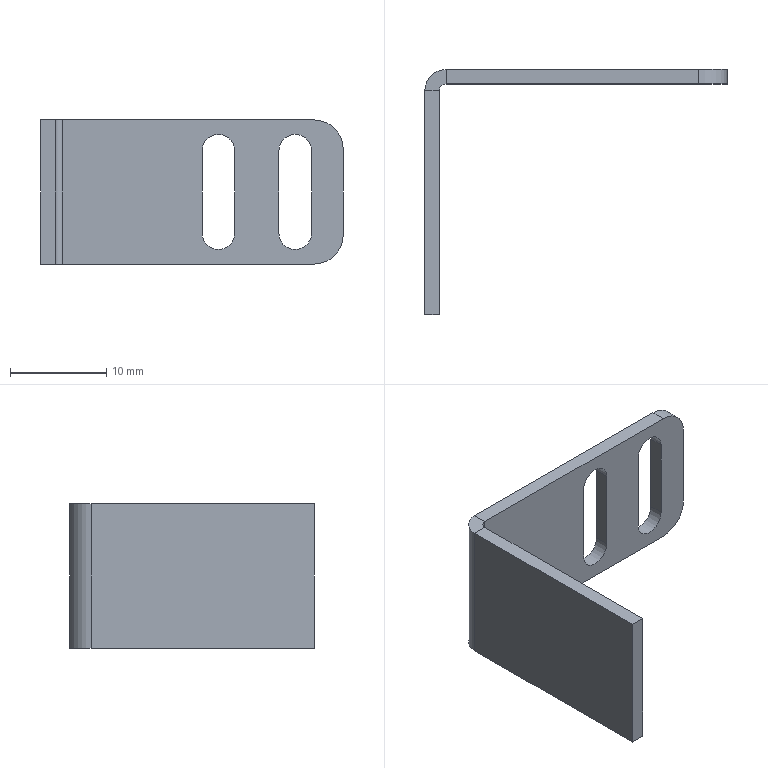Part | NX | features BREP 1 | 1 solid | 26 faces | box 31.5 x 25.5 x 15 mm | volume 1114 mm3 | plane 16 | cylinder 10 | commonest cylinder face diameters 3.4 x6 6 x2 1.473 x1 4.473 x1
STEP:
#1=CARTESIAN_POINT('',(26.7,0.,4.3));
#2=VERTEX_POINT('',#1);
#3=CARTESIAN_POINT('',(25.,0.,6.));
#4=VERTEX_POINT('',#3);
#5=CARTESIAN_POINT('',(25.,0.,4.3));
#6=DIRECTION('',(0.,-1.,0.));
#7=DIRECTION('',(0.,0.,-1.));
#8=AXIS2_PLACEMENT_3D('',#5,#6,#7);
#9=CIRCLE('',#8,1.7);
#10=EDGE_CURVE('',#2,#4,#9,.T.);
#11=ORIENTED_EDGE('',*,*,#10,.T.);
#12=CARTESIAN_POINT('',(25.,1.5,6.));
#13=VERTEX_POINT('',#12);
#14=CARTESIAN_POINT('',(25.,1.5,6.));
#15=DIRECTION('',(0.,1.,0.));
#16=VECTOR('',#15,1000.);
#17=LINE('',#14,#16);
#18=EDGE_CURVE('',#4,#13,#17,.T.);
#19=ORIENTED_EDGE('',*,*,#18,.T.);
#20=CARTESIAN_POINT('',(26.7,1.5,4.3));
#21=VERTEX_POINT('',#20);
#22=CARTESIAN_POINT('',(25.,1.5,4.3));
#23=DIRECTION('',(0.,1.,0.));
#24=DIRECTION('',(0.,0.,1.));
#25=AXIS2_PLACEMENT_3D('',#22,#23,#24);
#26=CIRCLE('',#25,1.7);
#27=EDGE_CURVE('',#13,#21,#26,.T.);
#28=ORIENTED_EDGE('',*,*,#27,.T.);
#29=CARTESIAN_POINT('',(26.7,-24.,4.3));
#30=DIRECTION('',(0.,-1.,0.));
#31=VECTOR('',#30,1000.);
#32=LINE('',#29,#31);
#33=EDGE_CURVE('',#21,#2,#32,.T.);
#34=ORIENTED_EDGE('',*,*,#33,.T.);
#35=EDGE_LOOP('',(#11,#19,#28,#34));
#36=FACE_BOUND('',#35,.T.);
#37=CARTESIAN_POINT('',(25.,1.5,4.3));
#38=DIRECTION('',(0.,1.,0.));
#39=DIRECTION('',(0.,0.,-1.));
#40=AXIS2_PLACEMENT_3D('',#37,#38,#39);
#41=CYLINDRICAL_SURFACE('',#40,1.7);
#42=ADVANCED_FACE('',(#36),#41,.F.);
#43=CARTESIAN_POINT('',(18.7,0.,4.3));
#44=VERTEX_POINT('',#43);
#45=CARTESIAN_POINT('',(17.,0.,6.));
#46=VERTEX_POINT('',#45);
#47=CARTESIAN_POINT('',(17.,0.,4.3));
#48=DIRECTION('',(0.,-1.,0.));
#49=DIRECTION('',(0.,0.,-1.));
#50=AXIS2_PLACEMENT_3D('',#47,#48,#49);
#51=CIRCLE('',#50,1.7);
#52=EDGE_CURVE('',#44,#46,#51,.T.);
#53=ORIENTED_EDGE('',*,*,#52,.T.);
#54=CARTESIAN_POINT('',(17.,1.5,6.));
#55=VERTEX_POINT('',#54);
#56=CARTESIAN_POINT('',(17.,1.5,6.));
#57=DIRECTION('',(0.,1.,0.));
#58=VECTOR('',#57,1000.);
#59=LINE('',#56,#58);
#60=EDGE_CURVE('',#46,#55,#59,.T.);
#61=ORIENTED_EDGE('',*,*,#60,.T.);
#62=CARTESIAN_POINT('',(18.7,1.5,4.3));
#63=VERTEX_POINT('',#62);
#64=CARTESIAN_POINT('',(17.,1.5,4.3));
#65=DIRECTION('',(0.,1.,0.));
#66=DIRECTION('',(0.,0.,1.));
#67=AXIS2_PLACEMENT_3D('',#64,#65,#66);
#68=CIRCLE('',#67,1.7);
#69=EDGE_CURVE('',#55,#63,#68,.T.);
#70=ORIENTED_EDGE('',*,*,#69,.T.);
#71=CARTESIAN_POINT('',(18.7,-24.,4.3));
#72=DIRECTION('',(0.,-1.,0.));
#73=VECTOR('',#72,1000.);
#74=LINE('',#71,#73);
#75=EDGE_CURVE('',#63,#44,#74,.T.);
#76=ORIENTED_EDGE('',*,*,#75,.T.);
#77=EDGE_LOOP('',(#53,#61,#70,#76));
#78=FACE_BOUND('',#77,.T.);
#79=CARTESIAN_POINT('',(17.,1.5,4.3));
#80=DIRECTION('',(0.,1.,0.));
#81=DIRECTION('',(0.,0.,-1.));
#82=AXIS2_PLACEMENT_3D('',#79,#80,#81);
#83=CYLINDRICAL_SURFACE('',#82,1.7);
#84=ADVANCED_FACE('',(#78),#83,.F.);
#85=CARTESIAN_POINT('',(0.,-0.7366,7.5));
#86=VERTEX_POINT('',#85);
#87=CARTESIAN_POINT('',(-1.5,-0.7366,7.5));
#88=VERTEX_POINT('',#87);
#89=CARTESIAN_POINT('',(0.,-0.7366,7.5));
#90=DIRECTION('',(-1.,0.,0.));
#91=VECTOR('',#90,1000.);
#92=LINE('',#89,#91);
#93=EDGE_CURVE('',#86,#88,#92,.T.);
#94=ORIENTED_EDGE('',*,*,#93,.F.);
#95=CARTESIAN_POINT('',(0.7366,0.,7.5));
#96=VERTEX_POINT('',#95);
#97=CARTESIAN_POINT('',(0.7366,-0.7366,7.5));
#98=DIRECTION('',(0.,0.,1.));
#99=DIRECTION('',(-1.,0.,0.));
#100=AXIS2_PLACEMENT_3D('',#97,#98,#99);
#101=CIRCLE('',#100,0.7366);
#102=EDGE_CURVE('',#96,#86,#101,.T.);
#103=ORIENTED_EDGE('',*,*,#102,.F.);
#104=CARTESIAN_POINT('',(0.7366,1.5,7.5));
#105=VERTEX_POINT('',#104);
#106=CARTESIAN_POINT('',(0.7366,1.5,7.5));
#107=DIRECTION('',(0.,-1.,0.));
#108=VECTOR('',#107,1000.);
#109=LINE('',#106,#108);
#110=EDGE_CURVE('',#105,#96,#109,.T.);
#111=ORIENTED_EDGE('',*,*,#110,.F.);
#112=CARTESIAN_POINT('',(0.7366,-0.7366,7.5));
#113=DIRECTION('',(0.,0.,1.));
#114=DIRECTION('',(1.,0.,0.));
#115=AXIS2_PLACEMENT_3D('',#112,#113,#114);
#116=CIRCLE('',#115,2.237);
#117=EDGE_CURVE('',#105,#88,#116,.T.);
#118=ORIENTED_EDGE('',*,*,#117,.T.);
#119=EDGE_LOOP('',(#94,#103,#111,#118));
#120=FACE_BOUND('',#119,.T.);
#121=CARTESIAN_POINT('',(0.,-0.7366,7.5));
#122=DIRECTION('',(0.,0.,1.));
#123=DIRECTION('',(-1.,0.,0.));
#124=AXIS2_PLACEMENT_3D('',#121,#122,#123);
#125=PLANE('',#124);
#126=ADVANCED_FACE('',(#120),#125,.T.);
#127=CARTESIAN_POINT('',(0.,-24.,7.5));
#128=VERTEX_POINT('',#127);
#129=CARTESIAN_POINT('',(0.,0.,7.5));
#130=DIRECTION('',(0.,-1.,0.));
#131=VECTOR('',#130,1000.);
#132=LINE('',#129,#131);
#133=EDGE_CURVE('',#86,#128,#132,.T.);
#134=ORIENTED_EDGE('',*,*,#133,.F.);
#135=ORIENTED_EDGE('',*,*,#93,.T.);
#136=CARTESIAN_POINT('',(-1.5,-24.,7.5));
#137=VERTEX_POINT('',#136);
#138=CARTESIAN_POINT('',(-1.5,0.,7.5));
#139=DIRECTION('',(0.,-1.,0.));
#140=VECTOR('',#139,1000.);
#141=LINE('',#138,#140);
#142=EDGE_CURVE('',#88,#137,#141,.T.);
#143=ORIENTED_EDGE('',*,*,#142,.T.);
#144=CARTESIAN_POINT('',(0.,-24.,7.5));
#145=DIRECTION('',(-1.,0.,0.));
#146=VECTOR('',#145,1000.);
#147=LINE('',#144,#146);
#148=EDGE_CURVE('',#128,#137,#147,.T.);
#149=ORIENTED_EDGE('',*,*,#148,.F.);
#150=EDGE_LOOP('',(#134,#135,#143,#149));
#151=FACE_BOUND('',#150,.T.);
#152=CARTESIAN_POINT('',(0.7366,1.5,7.5));
#153=DIRECTION('',(0.,0.,1.));
#154=DIRECTION('',(-1.,0.,0.));
#155=AXIS2_PLACEMENT_3D('',#152,#153,#154);
#156=PLANE('',#155);
#157=ADVANCED_FACE('',(#151),#156,.T.);
#158=CARTESIAN_POINT('',(0.7366,0.,-7.5));
#159=VERTEX_POINT('',#158);
#160=CARTESIAN_POINT('',(0.7366,1.5,-7.5));
#161=VERTEX_POINT('',#160);
#162=CARTESIAN_POINT('',(0.7366,0.,-7.5));
#163=DIRECTION('',(0.,1.,0.));
#164=VECTOR('',#163,1000.);
#165=LINE('',#162,#164);
#166=EDGE_CURVE('',#159,#161,#165,.T.);
#167=ORIENTED_EDGE('',*,*,#166,.F.);
#168=CARTESIAN_POINT('',(0.,-0.7366,-7.5));
#169=VERTEX_POINT('',#168);
#170=CARTESIAN_POINT('',(0.7366,-0.7366,-7.5));
#171=DIRECTION('',(0.,0.,1.));
#172=DIRECTION('',(-1.,0.,0.));
#173=AXIS2_PLACEMENT_3D('',#170,#171,#172);
#174=CIRCLE('',#173,0.7366);
#175=EDGE_CURVE('',#159,#169,#174,.T.);
#176=ORIENTED_EDGE('',*,*,#175,.T.);
#177=CARTESIAN_POINT('',(-1.5,-0.7366,-7.5));
#178=VERTEX_POINT('',#177);
#179=CARTESIAN_POINT('',(-1.5,-0.7366,-7.5));
#180=DIRECTION('',(1.,0.,0.));
#181=VECTOR('',#180,1000.);
#182=LINE('',#179,#181);
#183=EDGE_CURVE('',#178,#169,#182,.T.);
#184=ORIENTED_EDGE('',*,*,#183,.F.);
#185=CARTESIAN_POINT('',(0.7366,-0.7366,-7.5));
#186=DIRECTION('',(0.,0.,1.));
#187=DIRECTION('',(1.,0.,0.));
#188=AXIS2_PLACEMENT_3D('',#185,#186,#187);
#189=CIRCLE('',#188,2.237);
#190=EDGE_CURVE('',#161,#178,#189,.T.);
#191=ORIENTED_EDGE('',*,*,#190,.F.);
#192=EDGE_LOOP('',(#167,#176,#184,#191));
#193=FACE_BOUND('',#192,.T.);
#194=CARTESIAN_POINT('',(0.7366,0.,-7.5));
#195=DIRECTION('',(0.,0.,-1.));
#196=DIRECTION('',(1.,0.,0.));
#197=AXIS2_PLACEMENT_3D('',#194,#195,#196);
#198=PLANE('',#197);
#199=ADVANCED_FACE('',(#193),#198,.T.);
#200=CARTESIAN_POINT('',(27.,1.5,-7.5));
#201=VERTEX_POINT('',#200);
#202=CARTESIAN_POINT('',(0.,1.5,-7.5));
#203=DIRECTION('',(-1.,0.,0.));
#204=VECTOR('',#203,1000.);
#205=LINE('',#202,#204);
#206=EDGE_CURVE('',#201,#161,#205,.T.);
#207=ORIENTED_EDGE('',*,*,#206,.F.);
#208=CARTESIAN_POINT('',(27.,0.,-7.5));
#209=VERTEX_POINT('',#208);
#210=CARTESIAN_POINT('',(27.,-0.7366,-7.5));
#211=DIRECTION('',(0.,-1.,0.));
#212=VECTOR('',#211,1000.);
#213=LINE('',#210,#212);
#214=EDGE_CURVE('',#201,#209,#213,.T.);
#215=ORIENTED_EDGE('',*,*,#214,.T.);
#216=CARTESIAN_POINT('',(0.,0.,-7.5));
#217=DIRECTION('',(-1.,0.,0.));
#218=VECTOR('',#217,1000.);
#219=LINE('',#216,#218);
#220=EDGE_CURVE('',#209,#159,#219,.T.);
#221=ORIENTED_EDGE('',*,*,#220,.T.);
#222=ORIENTED_EDGE('',*,*,#166,.T.);
#223=EDGE_LOOP('',(#207,#215,#221,#222));
#224=FACE_BOUND('',#223,.T.);
#225=CARTESIAN_POINT('',(-1.5,-0.7366,-7.5));
#226=DIRECTION('',(0.,0.,-1.));
#227=DIRECTION('',(1.,0.,0.));
#228=AXIS2_PLACEMENT_3D('',#225,#226,#227);
#229=PLANE('',#228);
#230=ADVANCED_FACE('',(#224),#229,.T.);
#231=CARTESIAN_POINT('',(-1.5,-24.,-7.5));
#232=VERTEX_POINT('',#231);
#233=CARTESIAN_POINT('',(-1.5,0.,-7.5));
#234=DIRECTION('',(0.,-1.,0.));
#235=VECTOR('',#234,1000.);
#236=LINE('',#233,#235);
#237=EDGE_CURVE('',#178,#232,#236,.T.);
#238=ORIENTED_EDGE('',*,*,#237,.T.);
#239=CARTESIAN_POINT('',(-1.5,-24.,7.5));
#240=DIRECTION('',(0.,0.,-1.));
#241=VECTOR('',#240,1000.);
#242=LINE('',#239,#241);
#243=EDGE_CURVE('',#137,#232,#242,.T.);
#244=ORIENTED_EDGE('',*,*,#243,.F.);
#245=ORIENTED_EDGE('',*,*,#142,.F.);
#246=CARTESIAN_POINT('',(-1.5,-0.7366,7.5));
#247=DIRECTION('',(0.,0.,-1.));
#248=VECTOR('',#247,1000.);
#249=LINE('',#246,#248);
#250=EDGE_CURVE('',#88,#178,#249,.T.);
#251=ORIENTED_EDGE('',*,*,#250,.T.);
#252=EDGE_LOOP('',(#238,#244,#245,#251));
#253=FACE_BOUND('',#252,.T.);
#254=CARTESIAN_POINT('',(-1.5,0.,7.5));
#255=DIRECTION('',(1.,0.,0.));
#256=DIRECTION('',(0.,-1.,0.));
#257=AXIS2_PLACEMENT_3D('',#254,#255,#256);
#258=PLANE('',#257);
#259=ADVANCED_FACE('',(#253),#258,.F.);
#260=CARTESIAN_POINT('',(0.,-24.,-7.5));
#261=VERTEX_POINT('',#260);
#262=CARTESIAN_POINT('',(0.,-24.,-7.5));
#263=DIRECTION('',(-1.,0.,0.));
#264=VECTOR('',#263,1000.);
#265=LINE('',#262,#264);
#266=EDGE_CURVE('',#261,#232,#265,.T.);
#267=ORIENTED_EDGE('',*,*,#266,.F.);
#268=CARTESIAN_POINT('',(0.,-24.,7.5));
#269=DIRECTION('',(0.,0.,-1.));
#270=VECTOR('',#269,1000.);
#271=LINE('',#268,#270);
#272=EDGE_CURVE('',#128,#261,#271,.T.);
#273=ORIENTED_EDGE('',*,*,#272,.F.);
#274=ORIENTED_EDGE('',*,*,#148,.T.);
#275=ORIENTED_EDGE('',*,*,#243,.T.);
#276=EDGE_LOOP('',(#267,#273,#274,#275));
#277=FACE_BOUND('',#276,.T.);
#278=CARTESIAN_POINT('',(0.,-24.,7.5));
#279=DIRECTION('',(0.,-1.,0.));
#280=DIRECTION('',(0.,0.,1.));
#281=AXIS2_PLACEMENT_3D('',#278,#279,#280);
#282=PLANE('',#281);
#283=ADVANCED_FACE('',(#277),#282,.T.);
#284=CARTESIAN_POINT('',(0.,0.,-7.5));
#285=DIRECTION('',(0.,-1.,0.));
#286=VECTOR('',#285,1000.);
#287=LINE('',#284,#286);
#288=EDGE_CURVE('',#169,#261,#287,.T.);
#289=ORIENTED_EDGE('',*,*,#288,.F.);
#290=CARTESIAN_POINT('',(0.,-0.7366,7.5));
#291=DIRECTION('',(0.,0.,-1.));
#292=VECTOR('',#291,1000.);
#293=LINE('',#290,#292);
#294=EDGE_CURVE('',#86,#169,#293,.T.);
#295=ORIENTED_EDGE('',*,*,#294,.F.);
#296=ORIENTED_EDGE('',*,*,#133,.T.);
#297=ORIENTED_EDGE('',*,*,#272,.T.);
#298=EDGE_LOOP('',(#289,#295,#296,#297));
#299=FACE_BOUND('',#298,.T.);
#300=CARTESIAN_POINT('',(0.,0.,7.5));
#301=DIRECTION('',(1.,0.,0.));
#302=DIRECTION('',(0.,-1.,0.));
#303=AXIS2_PLACEMENT_3D('',#300,#301,#302);
#304=PLANE('',#303);
#305=ADVANCED_FACE('',(#299),#304,.T.);
#306=ORIENTED_EDGE('',*,*,#175,.F.);
#307=CARTESIAN_POINT('',(0.7366,0.,7.5));
#308=DIRECTION('',(0.,0.,-1.));
#309=VECTOR('',#308,1000.);
#310=LINE('',#307,#309);
#311=EDGE_CURVE('',#96,#159,#310,.T.);
#312=ORIENTED_EDGE('',*,*,#311,.F.);
#313=ORIENTED_EDGE('',*,*,#102,.T.);
#314=ORIENTED_EDGE('',*,*,#294,.T.);
#315=EDGE_LOOP('',(#306,#312,#313,#314));
#316=FACE_BOUND('',#315,.T.);
#317=CARTESIAN_POINT('',(0.7366,-0.7366,7.5));
#318=DIRECTION('',(0.,0.,-1.));
#319=DIRECTION('',(1.,0.,0.));
#320=AXIS2_PLACEMENT_3D('',#317,#318,#319);
#321=CYLINDRICAL_SURFACE('',#320,0.7366);
#322=ADVANCED_FACE('',(#316),#321,.F.);
#323=CARTESIAN_POINT('',(23.3,0.,4.3));
#324=VERTEX_POINT('',#323);
#325=CARTESIAN_POINT('',(23.3,0.,-4.3));
#326=VERTEX_POINT('',#325);
#327=CARTESIAN_POINT('',(23.3,0.,7.5));
#328=DIRECTION('',(0.,0.,-1.));
#329=VECTOR('',#328,1000.);
#330=LINE('',#327,#329);
#331=EDGE_CURVE('',#324,#326,#330,.T.);
#332=ORIENTED_EDGE('',*,*,#331,.F.);
#333=CARTESIAN_POINT('',(25.,0.,4.3));
#334=DIRECTION('',(0.,-1.,0.));
#335=DIRECTION('',(0.,0.,-1.));
#336=AXIS2_PLACEMENT_3D('',#333,#334,#335);
#337=CIRCLE('',#336,1.7);
#338=EDGE_CURVE('',#4,#324,#337,.T.);
#339=ORIENTED_EDGE('',*,*,#338,.F.);
#340=ORIENTED_EDGE('',*,*,#10,.F.);
#341=CARTESIAN_POINT('',(26.7,0.,-4.3));
#342=VERTEX_POINT('',#341);
#343=CARTESIAN_POINT('',(26.7,0.,7.5));
#344=DIRECTION('',(0.,0.,1.));
#345=VECTOR('',#344,1000.);
#346=LINE('',#343,#345);
#347=EDGE_CURVE('',#342,#2,#346,.T.);
#348=ORIENTED_EDGE('',*,*,#347,.F.);
#349=CARTESIAN_POINT('',(25.,0.,-4.3));
#350=DIRECTION('',(0.,-1.,0.));
#351=DIRECTION('',(0.,0.,-1.));
#352=AXIS2_PLACEMENT_3D('',#349,#350,#351);
#353=CIRCLE('',#352,1.7);
#354=EDGE_CURVE('',#326,#342,#353,.T.);
#355=ORIENTED_EDGE('',*,*,#354,.F.);
#356=EDGE_LOOP('',(#332,#339,#340,#348,#355));
#357=FACE_BOUND('',#356,.T.);
#358=CARTESIAN_POINT('',(15.3,0.,-4.3));
#359=VERTEX_POINT('',#358);
#360=CARTESIAN_POINT('',(18.7,0.,-4.3));
#361=VERTEX_POINT('',#360);
#362=CARTESIAN_POINT('',(17.,0.,-4.3));
#363=DIRECTION('',(0.,-1.,0.));
#364=DIRECTION('',(0.,0.,-1.));
#365=AXIS2_PLACEMENT_3D('',#362,#363,#364);
#366=CIRCLE('',#365,1.7);
#367=EDGE_CURVE('',#359,#361,#366,.T.);
#368=ORIENTED_EDGE('',*,*,#367,.F.);
#369=CARTESIAN_POINT('',(15.3,0.,4.3));
#370=VERTEX_POINT('',#369);
#371=CARTESIAN_POINT('',(15.3,0.,7.5));
#372=DIRECTION('',(0.,0.,-1.));
#373=VECTOR('',#372,1000.);
#374=LINE('',#371,#373);
#375=EDGE_CURVE('',#370,#359,#374,.T.);
#376=ORIENTED_EDGE('',*,*,#375,.F.);
#377=CARTESIAN_POINT('',(17.,0.,4.3));
#378=DIRECTION('',(0.,-1.,0.));
#379=DIRECTION('',(0.,0.,-1.));
#380=AXIS2_PLACEMENT_3D('',#377,#378,#379);
#381=CIRCLE('',#380,1.7);
#382=EDGE_CURVE('',#46,#370,#381,.T.);
#383=ORIENTED_EDGE('',*,*,#382,.F.);
#384=ORIENTED_EDGE('',*,*,#52,.F.);
#385=CARTESIAN_POINT('',(18.7,0.,7.5));
#386=DIRECTION('',(0.,0.,1.));
#387=VECTOR('',#386,1000.);
#388=LINE('',#385,#387);
#389=EDGE_CURVE('',#361,#44,#388,.T.);
#390=ORIENTED_EDGE('',*,*,#389,.F.);
#391=EDGE_LOOP('',(#368,#376,#383,#384,#390));
#392=FACE_BOUND('',#391,.T.);
#393=ORIENTED_EDGE('',*,*,#220,.F.);
#394=CARTESIAN_POINT('',(30.,0.,-4.5));
#395=VERTEX_POINT('',#394);
#396=CARTESIAN_POINT('',(27.,0.,-4.5));
#397=DIRECTION('',(0.,-1.,0.));
#398=DIRECTION('',(0.,0.,-1.));
#399=AXIS2_PLACEMENT_3D('',#396,#397,#398);
#400=CIRCLE('',#399,3.);
#401=EDGE_CURVE('',#209,#395,#400,.T.);
#402=ORIENTED_EDGE('',*,*,#401,.T.);
#403=CARTESIAN_POINT('',(30.,0.,4.5));
#404=VERTEX_POINT('',#403);
#405=CARTESIAN_POINT('',(30.,0.,7.5));
#406=DIRECTION('',(0.,0.,-1.));
#407=VECTOR('',#406,1000.);
#408=LINE('',#405,#407);
#409=EDGE_CURVE('',#404,#395,#408,.T.);
#410=ORIENTED_EDGE('',*,*,#409,.F.);
#411=CARTESIAN_POINT('',(27.,0.,7.5));
#412=VERTEX_POINT('',#411);
#413=CARTESIAN_POINT('',(27.,0.,4.5));
#414=DIRECTION('',(0.,-1.,0.));
#415=DIRECTION('',(0.,0.,-1.));
#416=AXIS2_PLACEMENT_3D('',#413,#414,#415);
#417=CIRCLE('',#416,3.);
#418=EDGE_CURVE('',#404,#412,#417,.T.);
#419=ORIENTED_EDGE('',*,*,#418,.T.);
#420=CARTESIAN_POINT('',(0.,0.,7.5));
#421=DIRECTION('',(-1.,0.,0.));
#422=VECTOR('',#421,1000.);
#423=LINE('',#420,#422);
#424=EDGE_CURVE('',#412,#96,#423,.T.);
#425=ORIENTED_EDGE('',*,*,#424,.T.);
#426=ORIENTED_EDGE('',*,*,#311,.T.);
#427=EDGE_LOOP('',(#393,#402,#410,#419,#425,#426));
#428=FACE_BOUND('',#427,.T.);
#429=CARTESIAN_POINT('',(0.,0.,7.5));
#430=DIRECTION('',(0.,-1.,0.));
#431=DIRECTION('',(0.,0.,1.));
#432=AXIS2_PLACEMENT_3D('',#429,#430,#431);
#433=PLANE('',#432);
#434=ADVANCED_FACE('',(#357,#392,#428),#433,.T.);
#435=ORIENTED_EDGE('',*,*,#409,.T.);
#436=CARTESIAN_POINT('',(30.,1.5,-4.5));
#437=VERTEX_POINT('',#436);
#438=CARTESIAN_POINT('',(30.,1.5,-4.5));
#439=DIRECTION('',(0.,1.,0.));
#440=VECTOR('',#439,1000.);
#441=LINE('',#438,#440);
#442=EDGE_CURVE('',#395,#437,#441,.T.);
#443=ORIENTED_EDGE('',*,*,#442,.T.);
#444=CARTESIAN_POINT('',(30.,1.5,4.5));
#445=VERTEX_POINT('',#444);
#446=CARTESIAN_POINT('',(30.,1.5,7.5));
#447=DIRECTION('',(0.,0.,-1.));
#448=VECTOR('',#447,1000.);
#449=LINE('',#446,#448);
#450=EDGE_CURVE('',#445,#437,#449,.T.);
#451=ORIENTED_EDGE('',*,*,#450,.F.);
#452=CARTESIAN_POINT('',(30.,0.,4.5));
#453=DIRECTION('',(0.,-1.,0.));
#454=VECTOR('',#453,1000.);
#455=LINE('',#452,#454);
#456=EDGE_CURVE('',#445,#404,#455,.T.);
#457=ORIENTED_EDGE('',*,*,#456,.T.);
#458=EDGE_LOOP('',(#435,#443,#451,#457));
#459=FACE_BOUND('',#458,.T.);
#460=CARTESIAN_POINT('',(30.,1.5,7.5));
#461=DIRECTION('',(1.,0.,0.));
#462=DIRECTION('',(0.,0.,1.));
#463=AXIS2_PLACEMENT_3D('',#460,#461,#462);
#464=PLANE('',#463);
#465=ADVANCED_FACE('',(#459),#464,.T.);
#466=CARTESIAN_POINT('',(26.7,1.5,-4.3));
#467=VERTEX_POINT('',#466);
#468=CARTESIAN_POINT('',(23.3,1.5,-4.3));
#469=VERTEX_POINT('',#468);
#470=CARTESIAN_POINT('',(25.,1.5,-4.3));
#471=DIRECTION('',(0.,1.,0.));
#472=DIRECTION('',(0.,0.,1.));
#473=AXIS2_PLACEMENT_3D('',#470,#471,#472);
#474=CIRCLE('',#473,1.7);
#475=EDGE_CURVE('',#467,#469,#474,.T.);
#476=ORIENTED_EDGE('',*,*,#475,.F.);
#477=CARTESIAN_POINT('',(26.7,1.5,4.3));
#478=DIRECTION('',(0.,0.,-1.));
#479=VECTOR('',#478,1000.);
#480=LINE('',#477,#479);
#481=EDGE_CURVE('',#21,#467,#480,.T.);
#482=ORIENTED_EDGE('',*,*,#481,.F.);
#483=ORIENTED_EDGE('',*,*,#27,.F.);
#484=CARTESIAN_POINT('',(23.3,1.5,4.3));
#485=VERTEX_POINT('',#484);
#486=CARTESIAN_POINT('',(25.,1.5,4.3));
#487=DIRECTION('',(0.,1.,0.));
#488=DIRECTION('',(0.,0.,1.));
#489=AXIS2_PLACEMENT_3D('',#486,#487,#488);
#490=CIRCLE('',#489,1.7);
#491=EDGE_CURVE('',#485,#13,#490,.T.);
#492=ORIENTED_EDGE('',*,*,#491,.F.);
#493=CARTESIAN_POINT('',(23.3,1.5,4.3));
#494=DIRECTION('',(0.,0.,-1.));
#495=VECTOR('',#494,1000.);
#496=LINE('',#493,#495);
#497=EDGE_CURVE('',#485,#469,#496,.T.);
#498=ORIENTED_EDGE('',*,*,#497,.T.);
#499=EDGE_LOOP('',(#476,#482,#483,#492,#498));
#500=FACE_BOUND('',#499,.T.);
#501=CARTESIAN_POINT('',(18.7,1.5,-4.3));
#502=VERTEX_POINT('',#501);
#503=CARTESIAN_POINT('',(15.3,1.5,-4.3));
#504=VERTEX_POINT('',#503);
#505=CARTESIAN_POINT('',(17.,1.5,-4.3));
#506=DIRECTION('',(0.,1.,0.));
#507=DIRECTION('',(0.,0.,1.));
#508=AXIS2_PLACEMENT_3D('',#505,#506,#507);
#509=CIRCLE('',#508,1.7);
#510=EDGE_CURVE('',#502,#504,#509,.T.);
#511=ORIENTED_EDGE('',*,*,#510,.F.);
#512=CARTESIAN_POINT('',(18.7,1.5,4.3));
#513=DIRECTION('',(0.,0.,-1.));
#514=VECTOR('',#513,1000.);
#515=LINE('',#512,#514);
#516=EDGE_CURVE('',#63,#502,#515,.T.);
#517=ORIENTED_EDGE('',*,*,#516,.F.);
#518=ORIENTED_EDGE('',*,*,#69,.F.);
#519=CARTESIAN_POINT('',(15.3,1.5,4.3));
#520=VERTEX_POINT('',#519);
#521=CARTESIAN_POINT('',(17.,1.5,4.3));
#522=DIRECTION('',(0.,1.,0.));
#523=DIRECTION('',(0.,0.,1.));
#524=AXIS2_PLACEMENT_3D('',#521,#522,#523);
#525=CIRCLE('',#524,1.7);
#526=EDGE_CURVE('',#520,#55,#525,.T.);
#527=ORIENTED_EDGE('',*,*,#526,.F.);
#528=CARTESIAN_POINT('',(15.3,1.5,4.3));
#529=DIRECTION('',(0.,0.,-1.));
#530=VECTOR('',#529,1000.);
#531=LINE('',#528,#530);
#532=EDGE_CURVE('',#520,#504,#531,.T.);
#533=ORIENTED_EDGE('',*,*,#532,.T.);
#534=EDGE_LOOP('',(#511,#517,#518,#527,#533));
#535=FACE_BOUND('',#534,.T.);
#536=ORIENTED_EDGE('',*,*,#450,.T.);
#537=CARTESIAN_POINT('',(27.,1.5,-4.5));
#538=DIRECTION('',(0.,1.,0.));
#539=DIRECTION('',(0.,0.,-1.));
#540=AXIS2_PLACEMENT_3D('',#537,#538,#539);
#541=CIRCLE('',#540,3.);
#542=EDGE_CURVE('',#437,#201,#541,.T.);
#543=ORIENTED_EDGE('',*,*,#542,.T.);
#544=ORIENTED_EDGE('',*,*,#206,.T.);
#545=CARTESIAN_POINT('',(0.7366,1.5,7.5));
#546=DIRECTION('',(0.,0.,-1.));
#547=VECTOR('',#546,1000.);
#548=LINE('',#545,#547);
#549=EDGE_CURVE('',#105,#161,#548,.T.);
#550=ORIENTED_EDGE('',*,*,#549,.F.);
#551=CARTESIAN_POINT('',(27.,1.5,7.5));
#552=VERTEX_POINT('',#551);
#553=CARTESIAN_POINT('',(0.,1.5,7.5));
#554=DIRECTION('',(-1.,0.,0.));
#555=VECTOR('',#554,1000.);
#556=LINE('',#553,#555);
#557=EDGE_CURVE('',#552,#105,#556,.T.);
#558=ORIENTED_EDGE('',*,*,#557,.F.);
#559=CARTESIAN_POINT('',(27.,1.5,4.5));
#560=DIRECTION('',(0.,1.,0.));
#561=DIRECTION('',(0.,0.,-1.));
#562=AXIS2_PLACEMENT_3D('',#559,#560,#561);
#563=CIRCLE('',#562,3.);
#564=EDGE_CURVE('',#552,#445,#563,.T.);
#565=ORIENTED_EDGE('',*,*,#564,.T.);
#566=EDGE_LOOP('',(#536,#543,#544,#550,#558,#565));
#567=FACE_BOUND('',#566,.T.);
#568=CARTESIAN_POINT('',(0.,1.5,7.5));
#569=DIRECTION('',(0.,-1.,0.));
#570=DIRECTION('',(0.,0.,1.));
#571=AXIS2_PLACEMENT_3D('',#568,#569,#570);
#572=PLANE('',#571);
#573=ADVANCED_FACE('',(#500,#535,#567),#572,.F.);
#574=ORIENTED_EDGE('',*,*,#190,.T.);
#575=ORIENTED_EDGE('',*,*,#250,.F.);
#576=ORIENTED_EDGE('',*,*,#117,.F.);
#577=ORIENTED_EDGE('',*,*,#549,.T.);
#578=EDGE_LOOP('',(#574,#575,#576,#577));
#579=FACE_BOUND('',#578,.T.);
#580=CARTESIAN_POINT('',(0.7366,-0.7366,7.5));
#581=DIRECTION('',(0.,0.,-1.));
#582=DIRECTION('',(1.,0.,0.));
#583=AXIS2_PLACEMENT_3D('',#580,#581,#582);
#584=CYLINDRICAL_SURFACE('',#583,2.237);
#585=ADVANCED_FACE('',(#579),#584,.T.);
#586=ORIENTED_EDGE('',*,*,#424,.F.);
#587=CARTESIAN_POINT('',(27.,1.5,7.5));
#588=DIRECTION('',(0.,1.,0.));
#589=VECTOR('',#588,1000.);
#590=LINE('',#587,#589);
#591=EDGE_CURVE('',#412,#552,#590,.T.);
#592=ORIENTED_EDGE('',*,*,#591,.T.);
#593=ORIENTED_EDGE('',*,*,#557,.T.);
#594=ORIENTED_EDGE('',*,*,#110,.T.);
#595=EDGE_LOOP('',(#586,#592,#593,#594));
#596=FACE_BOUND('',#595,.T.);
#597=CARTESIAN_POINT('',(0.7366,-0.7366,7.5));
#598=DIRECTION('',(0.,0.,-1.));
#599=DIRECTION('',(1.,0.,0.));
#600=AXIS2_PLACEMENT_3D('',#597,#598,#599);
#601=PLANE('',#600);
#602=ADVANCED_FACE('',(#596),#601,.F.);
#603=ORIENTED_EDGE('',*,*,#237,.F.);
#604=ORIENTED_EDGE('',*,*,#183,.T.);
#605=ORIENTED_EDGE('',*,*,#288,.T.);
#606=ORIENTED_EDGE('',*,*,#266,.T.);
#607=EDGE_LOOP('',(#603,#604,#605,#606));
#608=FACE_BOUND('',#607,.T.);
#609=CARTESIAN_POINT('',(0.7366,-0.7366,-7.5));
#610=DIRECTION('',(0.,0.,-1.));
#611=DIRECTION('',(1.,0.,0.));
#612=AXIS2_PLACEMENT_3D('',#609,#610,#611);
#613=PLANE('',#612);
#614=ADVANCED_FACE('',(#608),#613,.T.);
#615=ORIENTED_EDGE('',*,*,#367,.T.);
#616=CARTESIAN_POINT('',(18.7,-24.,-4.3));
#617=DIRECTION('',(0.,-1.,0.));
#618=VECTOR('',#617,1000.);
#619=LINE('',#616,#618);
#620=EDGE_CURVE('',#502,#361,#619,.T.);
#621=ORIENTED_EDGE('',*,*,#620,.F.);
#622=ORIENTED_EDGE('',*,*,#510,.T.);
#623=CARTESIAN_POINT('',(15.3,1.5,-4.3));
#624=DIRECTION('',(0.,1.,0.));
#625=VECTOR('',#624,1000.);
#626=LINE('',#623,#625);
#627=EDGE_CURVE('',#359,#504,#626,.T.);
#628=ORIENTED_EDGE('',*,*,#627,.F.);
#629=EDGE_LOOP('',(#615,#621,#622,#628));
#630=FACE_BOUND('',#629,.T.);
#631=CARTESIAN_POINT('',(17.,1.5,-4.3));
#632=DIRECTION('',(0.,1.,0.));
#633=DIRECTION('',(0.,0.,-1.));
#634=AXIS2_PLACEMENT_3D('',#631,#632,#633);
#635=CYLINDRICAL_SURFACE('',#634,1.7);
#636=ADVANCED_FACE('',(#630),#635,.F.);
#637=ORIENTED_EDGE('',*,*,#60,.F.);
#638=ORIENTED_EDGE('',*,*,#382,.T.);
#639=CARTESIAN_POINT('',(15.3,1.5,4.3));
#640=DIRECTION('',(0.,-1.,0.));
#641=VECTOR('',#640,1000.);
#642=LINE('',#639,#641);
#643=EDGE_CURVE('',#520,#370,#642,.T.);
#644=ORIENTED_EDGE('',*,*,#643,.F.);
#645=ORIENTED_EDGE('',*,*,#526,.T.);
#646=EDGE_LOOP('',(#637,#638,#644,#645));
#647=FACE_BOUND('',#646,.T.);
#648=CARTESIAN_POINT('',(17.,1.5,4.3));
#649=DIRECTION('',(0.,1.,0.));
#650=DIRECTION('',(0.,0.,-1.));
#651=AXIS2_PLACEMENT_3D('',#648,#649,#650);
#652=CYLINDRICAL_SURFACE('',#651,1.7);
#653=ADVANCED_FACE('',(#647),#652,.F.);
#654=ORIENTED_EDGE('',*,*,#375,.T.);
#655=ORIENTED_EDGE('',*,*,#627,.T.);
#656=ORIENTED_EDGE('',*,*,#532,.F.);
#657=ORIENTED_EDGE('',*,*,#643,.T.);
#658=EDGE_LOOP('',(#654,#655,#656,#657));
#659=FACE_BOUND('',#658,.T.);
#660=CARTESIAN_POINT('',(15.3,1.5,4.3));
#661=DIRECTION('',(-1.,0.,0.));
#662=DIRECTION('',(0.,0.,-1.));
#663=AXIS2_PLACEMENT_3D('',#660,#661,#662);
#664=PLANE('',#663);
#665=ADVANCED_FACE('',(#659),#664,.F.);
#666=ORIENTED_EDGE('',*,*,#389,.T.);
#667=ORIENTED_EDGE('',*,*,#75,.F.);
#668=ORIENTED_EDGE('',*,*,#516,.T.);
#669=ORIENTED_EDGE('',*,*,#620,.T.);
#670=EDGE_LOOP('',(#666,#667,#668,#669));
#671=FACE_BOUND('',#670,.T.);
#672=CARTESIAN_POINT('',(18.7,-24.,4.3));
#673=DIRECTION('',(1.,0.,0.));
#674=DIRECTION('',(0.,-1.,0.));
#675=AXIS2_PLACEMENT_3D('',#672,#673,#674);
#676=PLANE('',#675);
#677=ADVANCED_FACE('',(#671),#676,.F.);
#678=ORIENTED_EDGE('',*,*,#354,.T.);
#679=CARTESIAN_POINT('',(26.7,-24.,-4.3));
#680=DIRECTION('',(0.,-1.,0.));
#681=VECTOR('',#680,1000.);
#682=LINE('',#679,#681);
#683=EDGE_CURVE('',#467,#342,#682,.T.);
#684=ORIENTED_EDGE('',*,*,#683,.F.);
#685=ORIENTED_EDGE('',*,*,#475,.T.);
#686=CARTESIAN_POINT('',(23.3,1.5,-4.3));
#687=DIRECTION('',(0.,1.,0.));
#688=VECTOR('',#687,1000.);
#689=LINE('',#686,#688);
#690=EDGE_CURVE('',#326,#469,#689,.T.);
#691=ORIENTED_EDGE('',*,*,#690,.F.);
#692=EDGE_LOOP('',(#678,#684,#685,#691));
#693=FACE_BOUND('',#692,.T.);
#694=CARTESIAN_POINT('',(25.,1.5,-4.3));
#695=DIRECTION('',(0.,1.,0.));
#696=DIRECTION('',(0.,0.,-1.));
#697=AXIS2_PLACEMENT_3D('',#694,#695,#696);
#698=CYLINDRICAL_SURFACE('',#697,1.7);
#699=ADVANCED_FACE('',(#693),#698,.F.);
#700=ORIENTED_EDGE('',*,*,#18,.F.);
#701=ORIENTED_EDGE('',*,*,#338,.T.);
#702=CARTESIAN_POINT('',(23.3,1.5,4.3));
#703=DIRECTION('',(0.,-1.,0.));
#704=VECTOR('',#703,1000.);
#705=LINE('',#702,#704);
#706=EDGE_CURVE('',#485,#324,#705,.T.);
#707=ORIENTED_EDGE('',*,*,#706,.F.);
#708=ORIENTED_EDGE('',*,*,#491,.T.);
#709=EDGE_LOOP('',(#700,#701,#707,#708));
#710=FACE_BOUND('',#709,.T.);
#711=CARTESIAN_POINT('',(25.,1.5,4.3));
#712=DIRECTION('',(0.,1.,0.));
#713=DIRECTION('',(0.,0.,-1.));
#714=AXIS2_PLACEMENT_3D('',#711,#712,#713);
#715=CYLINDRICAL_SURFACE('',#714,1.7);
#716=ADVANCED_FACE('',(#710),#715,.F.);
#717=ORIENTED_EDGE('',*,*,#331,.T.);
#718=ORIENTED_EDGE('',*,*,#690,.T.);
#719=ORIENTED_EDGE('',*,*,#497,.F.);
#720=ORIENTED_EDGE('',*,*,#706,.T.);
#721=EDGE_LOOP('',(#717,#718,#719,#720));
#722=FACE_BOUND('',#721,.T.);
#723=CARTESIAN_POINT('',(23.3,1.5,4.3));
#724=DIRECTION('',(-1.,0.,0.));
#725=DIRECTION('',(0.,0.,-1.));
#726=AXIS2_PLACEMENT_3D('',#723,#724,#725);
#727=PLANE('',#726);
#728=ADVANCED_FACE('',(#722),#727,.F.);
#729=ORIENTED_EDGE('',*,*,#347,.T.);
#730=ORIENTED_EDGE('',*,*,#33,.F.);
#731=ORIENTED_EDGE('',*,*,#481,.T.);
#732=ORIENTED_EDGE('',*,*,#683,.T.);
#733=EDGE_LOOP('',(#729,#730,#731,#732));
#734=FACE_BOUND('',#733,.T.);
#735=CARTESIAN_POINT('',(26.7,-24.,4.3));
#736=DIRECTION('',(1.,0.,0.));
#737=DIRECTION('',(0.,-1.,0.));
#738=AXIS2_PLACEMENT_3D('',#735,#736,#737);
#739=PLANE('',#738);
#740=ADVANCED_FACE('',(#734),#739,.F.);
#741=ORIENTED_EDGE('',*,*,#542,.F.);
#742=ORIENTED_EDGE('',*,*,#442,.F.);
#743=ORIENTED_EDGE('',*,*,#401,.F.);
#744=ORIENTED_EDGE('',*,*,#214,.F.);
#745=EDGE_LOOP('',(#741,#742,#743,#744));
#746=FACE_BOUND('',#745,.T.);
#747=CARTESIAN_POINT('',(27.,-0.7366,-4.5));
#748=DIRECTION('',(0.,-1.,0.));
#749=DIRECTION('',(0.,0.,1.));
#750=AXIS2_PLACEMENT_3D('',#747,#748,#749);
#751=CYLINDRICAL_SURFACE('',#750,3.);
#752=ADVANCED_FACE('',(#746),#751,.T.);
#753=ORIENTED_EDGE('',*,*,#564,.F.);
#754=ORIENTED_EDGE('',*,*,#591,.F.);
#755=ORIENTED_EDGE('',*,*,#418,.F.);
#756=ORIENTED_EDGE('',*,*,#456,.F.);
#757=EDGE_LOOP('',(#753,#754,#755,#756));
#758=FACE_BOUND('',#757,.T.);
#759=CARTESIAN_POINT('',(27.,1.5,4.5));
#760=DIRECTION('',(0.,1.,0.));
#761=DIRECTION('',(0.,0.,-1.));
#762=AXIS2_PLACEMENT_3D('',#759,#760,#761);
#763=CYLINDRICAL_SURFACE('',#762,3.);
#764=ADVANCED_FACE('',(#758),#763,.T.);
#765=CLOSED_SHELL('',(#42,#84,#126,#157,#199,#230,#259,#283,#305,#322,#434,#465,#573,#585,#602,#614,#636,#653,#665,#677,#699,#716,#728,#740,#752,#764));
#766=MANIFOLD_SOLID_BREP('',#765);
#767=(LENGTH_UNIT()NAMED_UNIT(*)SI_UNIT(.MILLI.,.METRE.));
#768=UNCERTAINTY_MEASURE_WITH_UNIT(LENGTH_MEASURE(0.00001),#767,'','');
#769=(NAMED_UNIT(*)PLANE_ANGLE_UNIT()SI_UNIT($,.RADIAN.));
#770=(NAMED_UNIT(*)SI_UNIT($,.STERADIAN.)SOLID_ANGLE_UNIT());
#771=(GEOMETRIC_REPRESENTATION_CONTEXT(3)GLOBAL_UNCERTAINTY_ASSIGNED_CONTEXT((#768))GLOBAL_UNIT_ASSIGNED_CONTEXT((#767,#769,#770))REPRESENTATION_CONTEXT('',''));
#772=ADVANCED_BREP_SHAPE_REPRESENTATION('',(#766),#771);